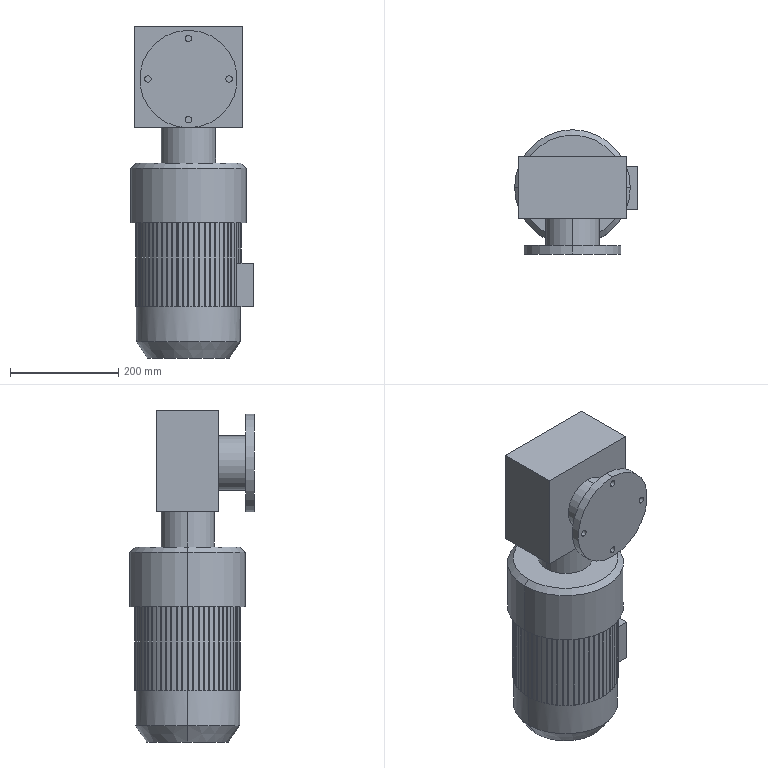Part | SolidWorks | features ICE 11, Chamfer 2, CirPattern 1, Extrusion 1 | 1 solid | 379 faces | box 226.9 x 230.198 x 613 mm | volume 16882473 mm3 | plane 297 | cylinder 78 | cone 4 | commonest cylinder face diameters 195 x60 12 x8 100 x4 180 x2 192 x2 213.8 x2